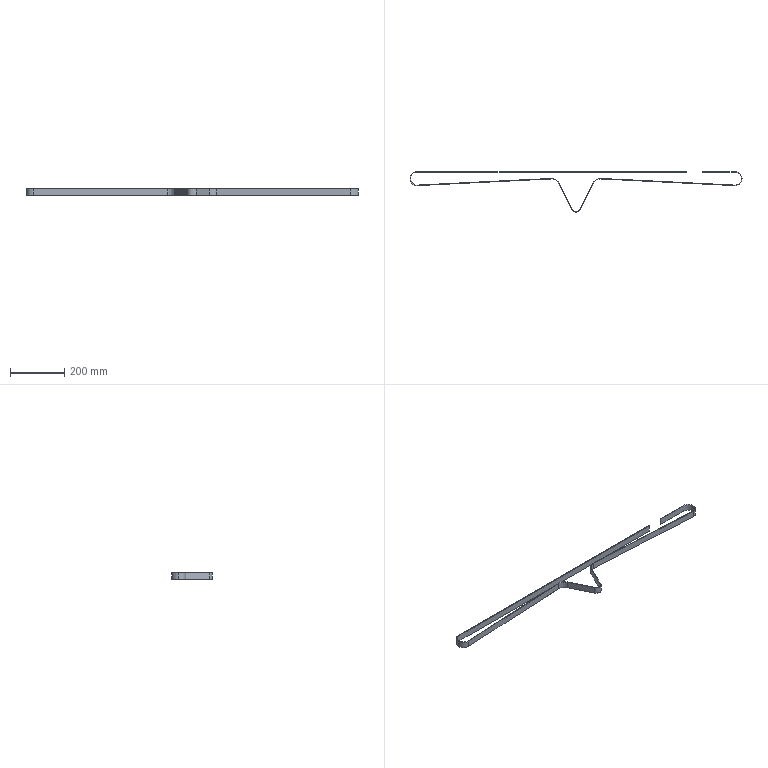Part | SolidWorks | features BaseBody 1 | 1 solid | 28 faces | box 1221 x 148.8 x 24 mm | volume 123601 mm3 | plane 16 | cylinder 12 | commonest cylinder face diameters 47 x3 51 x3 60 x2 64 x2 31 x1 35 x1
STEP:
#1=CARTESIAN_POINT('',(-1151.5,-71.7,12.));
#2=VERTEX_POINT('',#1);
#3=CARTESIAN_POINT('',(-1128.,-48.2,12.));
#4=VERTEX_POINT('',#3);
#5=CARTESIAN_POINT('',(-1128.,-71.7,12.));
#6=DIRECTION('',(0.,0.,-1.));
#7=DIRECTION('',(-1.,0.,0.));
#8=AXIS2_PLACEMENT_3D('',#5,#6,#7);
#9=CIRCLE('',#8,23.5);
#10=EDGE_CURVE('',#2,#4,#9,.T.);
#11=ORIENTED_EDGE('',*,*,#10,.F.);
#12=CARTESIAN_POINT('',(-1151.5,-71.7,-12.));
#13=VERTEX_POINT('',#12);
#14=CARTESIAN_POINT('',(-1151.5,-71.7,12.));
#15=DIRECTION('',(0.,0.,-1.));
#16=VECTOR('',#15,1000.);
#17=LINE('',#14,#16);
#18=EDGE_CURVE('',#2,#13,#17,.T.);
#19=ORIENTED_EDGE('',*,*,#18,.T.);
#20=CARTESIAN_POINT('',(-1128.,-48.2,-12.));
#21=VERTEX_POINT('',#20);
#22=CARTESIAN_POINT('',(-1128.,-71.7,-12.));
#23=DIRECTION('',(0.,0.,-1.));
#24=DIRECTION('',(-1.,0.,0.));
#25=AXIS2_PLACEMENT_3D('',#22,#23,#24);
#26=CIRCLE('',#25,23.5);
#27=EDGE_CURVE('',#13,#21,#26,.T.);
#28=ORIENTED_EDGE('',*,*,#27,.T.);
#29=CARTESIAN_POINT('',(-1128.,-48.2,12.));
#30=DIRECTION('',(0.,0.,-1.));
#31=VECTOR('',#30,1000.);
#32=LINE('',#29,#31);
#33=EDGE_CURVE('',#4,#21,#32,.T.);
#34=ORIENTED_EDGE('',*,*,#33,.F.);
#35=EDGE_LOOP('',(#11,#19,#28,#34));
#36=FACE_OUTER_BOUND('',#35,.T.);
#37=CARTESIAN_POINT('',(-1128.,-71.7,12.));
#38=DIRECTION('',(0.,0.,-1.));
#39=DIRECTION('',(-1.,0.,0.));
#40=AXIS2_PLACEMENT_3D('',#37,#38,#39);
#41=CYLINDRICAL_SURFACE('',#40,23.5);
#42=ADVANCED_FACE('',(#36),#41,.F.);
#43=CARTESIAN_POINT('',(-1153.5,-71.7,12.));
#44=VERTEX_POINT('',#43);
#45=CARTESIAN_POINT('',(-1126.726,-97.168,12.));
#46=VERTEX_POINT('',#45);
#47=CARTESIAN_POINT('',(-1128.,-71.7,12.));
#48=DIRECTION('',(0.,0.,1.));
#49=DIRECTION('',(1.,0.,0.));
#50=AXIS2_PLACEMENT_3D('',#47,#48,#49);
#51=CIRCLE('',#50,25.5);
#52=EDGE_CURVE('',#44,#46,#51,.T.);
#53=ORIENTED_EDGE('',*,*,#52,.F.);
#54=CARTESIAN_POINT('',(-1153.5,-71.7,-12.));
#55=VERTEX_POINT('',#54);
#56=CARTESIAN_POINT('',(-1153.5,-71.7,12.));
#57=DIRECTION('',(0.,0.,-1.));
#58=VECTOR('',#57,1000.);
#59=LINE('',#56,#58);
#60=EDGE_CURVE('',#44,#55,#59,.T.);
#61=ORIENTED_EDGE('',*,*,#60,.T.);
#62=CARTESIAN_POINT('',(-1126.726,-97.168,-12.));
#63=VERTEX_POINT('',#62);
#64=CARTESIAN_POINT('',(-1128.,-71.7,-12.));
#65=DIRECTION('',(0.,0.,1.));
#66=DIRECTION('',(1.,0.,0.));
#67=AXIS2_PLACEMENT_3D('',#64,#65,#66);
#68=CIRCLE('',#67,25.5);
#69=EDGE_CURVE('',#55,#63,#68,.T.);
#70=ORIENTED_EDGE('',*,*,#69,.T.);
#71=CARTESIAN_POINT('',(-1126.726,-97.168,12.));
#72=DIRECTION('',(0.,0.,-1.));
#73=VECTOR('',#72,1000.);
#74=LINE('',#71,#73);
#75=EDGE_CURVE('',#46,#63,#74,.T.);
#76=ORIENTED_EDGE('',*,*,#75,.F.);
#77=EDGE_LOOP('',(#53,#61,#70,#76));
#78=FACE_OUTER_BOUND('',#77,.T.);
#79=CARTESIAN_POINT('',(-1128.,-71.7,12.));
#80=DIRECTION('',(0.,0.,-1.));
#81=DIRECTION('',(-1.,0.,0.));
#82=AXIS2_PLACEMENT_3D('',#79,#80,#81);
#83=CYLINDRICAL_SURFACE('',#82,25.5);
#84=ADVANCED_FACE('',(#78),#83,.T.);
#85=CARTESIAN_POINT('',(-138.,-46.2,12.));
#86=VERTEX_POINT('',#85);
#87=CARTESIAN_POINT('',(-1128.,-46.2,12.));
#88=VERTEX_POINT('',#87);
#89=CARTESIAN_POINT('',(-1128.,-46.2,12.));
#90=DIRECTION('',(-1.,0.,0.));
#91=VECTOR('',#90,1000.);
#92=LINE('',#89,#91);
#93=EDGE_CURVE('',#86,#88,#92,.T.);
#94=ORIENTED_EDGE('',*,*,#93,.F.);
#95=CARTESIAN_POINT('',(-138.,-46.2,-12.));
#96=VERTEX_POINT('',#95);
#97=CARTESIAN_POINT('',(-138.,-46.2,12.));
#98=DIRECTION('',(0.,0.,1.));
#99=VECTOR('',#98,1000.);
#100=LINE('',#97,#99);
#101=EDGE_CURVE('',#96,#86,#100,.T.);
#102=ORIENTED_EDGE('',*,*,#101,.F.);
#103=CARTESIAN_POINT('',(-1128.,-46.2,-12.));
#104=VERTEX_POINT('',#103);
#105=CARTESIAN_POINT('',(-1128.,-46.2,-12.));
#106=DIRECTION('',(-1.,0.,0.));
#107=VECTOR('',#106,1000.);
#108=LINE('',#105,#107);
#109=EDGE_CURVE('',#96,#104,#108,.T.);
#110=ORIENTED_EDGE('',*,*,#109,.T.);
#111=CARTESIAN_POINT('',(-1128.,-46.2,12.));
#112=DIRECTION('',(0.,0.,-1.));
#113=VECTOR('',#112,1000.);
#114=LINE('',#111,#113);
#115=EDGE_CURVE('',#88,#104,#114,.T.);
#116=ORIENTED_EDGE('',*,*,#115,.F.);
#117=EDGE_LOOP('',(#94,#102,#110,#116));
#118=FACE_OUTER_BOUND('',#117,.T.);
#119=CARTESIAN_POINT('',(-1128.,-46.2,12.));
#120=DIRECTION('',(0.,-1.,0.));
#121=DIRECTION('',(0.,0.,-1.));
#122=AXIS2_PLACEMENT_3D('',#119,#120,#121);
#123=PLANE('',#122);
#124=ADVANCED_FACE('',(#118),#123,.F.);
#125=CARTESIAN_POINT('',(-138.,-48.2,12.));
#126=VERTEX_POINT('',#125);
#127=CARTESIAN_POINT('',(-138.,-48.2,-12.));
#128=VERTEX_POINT('',#127);
#129=CARTESIAN_POINT('',(-138.,-48.2,12.));
#130=DIRECTION('',(0.,0.,-1.));
#131=VECTOR('',#130,1000.);
#132=LINE('',#129,#131);
#133=EDGE_CURVE('',#126,#128,#132,.T.);
#134=ORIENTED_EDGE('',*,*,#133,.F.);
#135=CARTESIAN_POINT('',(-1128.,-48.2,12.));
#136=DIRECTION('',(1.,0.,0.));
#137=VECTOR('',#136,1000.);
#138=LINE('',#135,#137);
#139=EDGE_CURVE('',#4,#126,#138,.T.);
#140=ORIENTED_EDGE('',*,*,#139,.F.);
#141=ORIENTED_EDGE('',*,*,#33,.T.);
#142=CARTESIAN_POINT('',(-1128.,-48.2,-12.));
#143=DIRECTION('',(1.,0.,0.));
#144=VECTOR('',#143,1000.);
#145=LINE('',#142,#144);
#146=EDGE_CURVE('',#21,#128,#145,.T.);
#147=ORIENTED_EDGE('',*,*,#146,.T.);
#148=EDGE_LOOP('',(#134,#140,#141,#147));
#149=FACE_OUTER_BOUND('',#148,.T.);
#150=CARTESIAN_POINT('',(-1128.,-48.2,12.));
#151=DIRECTION('',(0.,-1.,0.));
#152=DIRECTION('',(0.,0.,-1.));
#153=AXIS2_PLACEMENT_3D('',#150,#151,#152);
#154=PLANE('',#153);
#155=ADVANCED_FACE('',(#149),#154,.T.);
#156=CARTESIAN_POINT('',(40.726,-97.168,-12.));
#157=VERTEX_POINT('',#156);
#158=CARTESIAN_POINT('',(42.,-46.2,-12.));
#159=VERTEX_POINT('',#158);
#160=CARTESIAN_POINT('',(42.,-71.7,-12.));
#161=DIRECTION('',(0.,0.,1.));
#162=DIRECTION('',(1.,0.,0.));
#163=AXIS2_PLACEMENT_3D('',#160,#161,#162);
#164=CIRCLE('',#163,25.5);
#165=EDGE_CURVE('',#157,#159,#164,.T.);
#166=ORIENTED_EDGE('',*,*,#165,.T.);
#167=CARTESIAN_POINT('',(42.,-46.2,12.));
#168=VERTEX_POINT('',#167);
#169=CARTESIAN_POINT('',(42.,-46.2,12.));
#170=DIRECTION('',(0.,0.,-1.));
#171=VECTOR('',#170,1000.);
#172=LINE('',#169,#171);
#173=EDGE_CURVE('',#168,#159,#172,.T.);
#174=ORIENTED_EDGE('',*,*,#173,.F.);
#175=CARTESIAN_POINT('',(40.726,-97.168,12.));
#176=VERTEX_POINT('',#175);
#177=CARTESIAN_POINT('',(42.,-71.7,12.));
#178=DIRECTION('',(0.,0.,1.));
#179=DIRECTION('',(1.,0.,0.));
#180=AXIS2_PLACEMENT_3D('',#177,#178,#179);
#181=CIRCLE('',#180,25.5);
#182=EDGE_CURVE('',#176,#168,#181,.T.);
#183=ORIENTED_EDGE('',*,*,#182,.F.);
#184=CARTESIAN_POINT('',(40.726,-97.168,12.));
#185=DIRECTION('',(0.,0.,-1.));
#186=VECTOR('',#185,1000.);
#187=LINE('',#184,#186);
#188=EDGE_CURVE('',#176,#157,#187,.T.);
#189=ORIENTED_EDGE('',*,*,#188,.T.);
#190=EDGE_LOOP('',(#166,#174,#183,#189));
#191=FACE_OUTER_BOUND('',#190,.T.);
#192=CARTESIAN_POINT('',(42.,-71.7,12.));
#193=DIRECTION('',(0.,0.,-1.));
#194=DIRECTION('',(-1.,0.,0.));
#195=AXIS2_PLACEMENT_3D('',#192,#193,#194);
#196=CYLINDRICAL_SURFACE('',#195,25.5);
#197=ADVANCED_FACE('',(#191),#196,.T.);
#198=CARTESIAN_POINT('',(-78.,-46.2,-12.));
#199=VERTEX_POINT('',#198);
#200=CARTESIAN_POINT('',(-1128.,-46.2,-12.));
#201=DIRECTION('',(-1.,0.,0.));
#202=VECTOR('',#201,1000.);
#203=LINE('',#200,#202);
#204=EDGE_CURVE('',#159,#199,#203,.T.);
#205=ORIENTED_EDGE('',*,*,#204,.T.);
#206=CARTESIAN_POINT('',(-78.,-46.2,12.));
#207=VERTEX_POINT('',#206);
#208=CARTESIAN_POINT('',(-78.,-46.2,12.));
#209=DIRECTION('',(0.,0.,-1.));
#210=VECTOR('',#209,1000.);
#211=LINE('',#208,#210);
#212=EDGE_CURVE('',#207,#199,#211,.T.);
#213=ORIENTED_EDGE('',*,*,#212,.F.);
#214=CARTESIAN_POINT('',(-1128.,-46.2,12.));
#215=DIRECTION('',(-1.,0.,0.));
#216=VECTOR('',#215,1000.);
#217=LINE('',#214,#216);
#218=EDGE_CURVE('',#168,#207,#217,.T.);
#219=ORIENTED_EDGE('',*,*,#218,.F.);
#220=ORIENTED_EDGE('',*,*,#173,.T.);
#221=EDGE_LOOP('',(#205,#213,#219,#220));
#222=FACE_OUTER_BOUND('',#221,.T.);
#223=CARTESIAN_POINT('',(-1128.,-46.2,12.));
#224=DIRECTION('',(0.,-1.,0.));
#225=DIRECTION('',(0.,0.,-1.));
#226=AXIS2_PLACEMENT_3D('',#223,#224,#225);
#227=PLANE('',#226);
#228=ADVANCED_FACE('',(#222),#227,.F.);
#229=ORIENTED_EDGE('',*,*,#60,.F.);
#230=CARTESIAN_POINT('',(-1128.,-71.7,12.));
#231=DIRECTION('',(0.,0.,1.));
#232=DIRECTION('',(1.,0.,0.));
#233=AXIS2_PLACEMENT_3D('',#230,#231,#232);
#234=CIRCLE('',#233,25.5);
#235=EDGE_CURVE('',#88,#44,#234,.T.);
#236=ORIENTED_EDGE('',*,*,#235,.F.);
#237=ORIENTED_EDGE('',*,*,#115,.T.);
#238=CARTESIAN_POINT('',(-1128.,-71.7,-12.));
#239=DIRECTION('',(0.,0.,1.));
#240=DIRECTION('',(1.,0.,0.));
#241=AXIS2_PLACEMENT_3D('',#238,#239,#240);
#242=CIRCLE('',#241,25.5);
#243=EDGE_CURVE('',#104,#55,#242,.T.);
#244=ORIENTED_EDGE('',*,*,#243,.T.);
#245=EDGE_LOOP('',(#229,#236,#237,#244));
#246=FACE_OUTER_BOUND('',#245,.T.);
#247=CARTESIAN_POINT('',(-1128.,-71.7,12.));
#248=DIRECTION('',(0.,0.,-1.));
#249=DIRECTION('',(-1.,0.,0.));
#250=AXIS2_PLACEMENT_3D('',#247,#248,#249);
#251=CYLINDRICAL_SURFACE('',#250,25.5);
#252=ADVANCED_FACE('',(#246),#251,.T.);
#253=CARTESIAN_POINT('',(-634.499,-72.537,-12.));
#254=VERTEX_POINT('',#253);
#255=CARTESIAN_POINT('',(-1126.726,-97.168,-12.));
#256=DIRECTION('',(0.9988,0.04998,0.));
#257=VECTOR('',#256,1000.);
#258=LINE('',#255,#257);
#259=EDGE_CURVE('',#63,#254,#258,.T.);
#260=ORIENTED_EDGE('',*,*,#259,.T.);
#261=CARTESIAN_POINT('',(-634.499,-72.537,12.));
#262=VERTEX_POINT('',#261);
#263=CARTESIAN_POINT('',(-634.499,-72.537,12.));
#264=DIRECTION('',(0.,0.,-1.));
#265=VECTOR('',#264,1000.);
#266=LINE('',#263,#265);
#267=EDGE_CURVE('',#262,#254,#266,.T.);
#268=ORIENTED_EDGE('',*,*,#267,.F.);
#269=CARTESIAN_POINT('',(-1126.726,-97.168,12.));
#270=DIRECTION('',(0.9988,0.04998,0.));
#271=VECTOR('',#270,1000.);
#272=LINE('',#269,#271);
#273=EDGE_CURVE('',#46,#262,#272,.T.);
#274=ORIENTED_EDGE('',*,*,#273,.F.);
#275=ORIENTED_EDGE('',*,*,#75,.T.);
#276=EDGE_LOOP('',(#260,#268,#274,#275));
#277=FACE_OUTER_BOUND('',#276,.T.);
#278=CARTESIAN_POINT('',(-1126.726,-97.168,12.));
#279=DIRECTION('',(-0.04998,0.9988,0.));
#280=DIRECTION('',(-0.9988,-0.04998,0.));
#281=AXIS2_PLACEMENT_3D('',#278,#279,#280);
#282=PLANE('',#281);
#283=ADVANCED_FACE('',(#277),#282,.F.);
#284=CARTESIAN_POINT('',(-606.1,-89.22,-12.));
#285=VERTEX_POINT('',#284);
#286=CARTESIAN_POINT('',(-633.,-102.5,-12.));
#287=DIRECTION('',(0.,0.,-1.));
#288=DIRECTION('',(1.,0.,0.));
#289=AXIS2_PLACEMENT_3D('',#286,#287,#288);
#290=CIRCLE('',#289,30.);
#291=EDGE_CURVE('',#254,#285,#290,.T.);
#292=ORIENTED_EDGE('',*,*,#291,.T.);
#293=CARTESIAN_POINT('',(-606.1,-89.22,12.));
#294=VERTEX_POINT('',#293);
#295=CARTESIAN_POINT('',(-606.1,-89.22,12.));
#296=DIRECTION('',(0.,0.,-1.));
#297=VECTOR('',#296,1000.);
#298=LINE('',#295,#297);
#299=EDGE_CURVE('',#294,#285,#298,.T.);
#300=ORIENTED_EDGE('',*,*,#299,.F.);
#301=CARTESIAN_POINT('',(-633.,-102.5,12.));
#302=DIRECTION('',(0.,0.,-1.));
#303=DIRECTION('',(1.,0.,0.));
#304=AXIS2_PLACEMENT_3D('',#301,#302,#303);
#305=CIRCLE('',#304,30.);
#306=EDGE_CURVE('',#262,#294,#305,.T.);
#307=ORIENTED_EDGE('',*,*,#306,.F.);
#308=ORIENTED_EDGE('',*,*,#267,.T.);
#309=EDGE_LOOP('',(#292,#300,#307,#308));
#310=FACE_OUTER_BOUND('',#309,.T.);
#311=CARTESIAN_POINT('',(-633.,-102.5,12.));
#312=DIRECTION('',(0.,0.,-1.));
#313=DIRECTION('',(-1.,0.,0.));
#314=AXIS2_PLACEMENT_3D('',#311,#312,#313);
#315=CYLINDRICAL_SURFACE('',#314,30.);
#316=ADVANCED_FACE('',(#310),#315,.F.);
#317=CARTESIAN_POINT('',(-558.692,-185.247,-12.));
#318=VERTEX_POINT('',#317);
#319=CARTESIAN_POINT('',(-606.1,-89.22,-12.));
#320=DIRECTION('',(0.4427,-0.8967,0.));
#321=VECTOR('',#320,1000.);
#322=LINE('',#319,#321);
#323=EDGE_CURVE('',#285,#318,#322,.T.);
#324=ORIENTED_EDGE('',*,*,#323,.T.);
#325=CARTESIAN_POINT('',(-558.692,-185.247,12.));
#326=VERTEX_POINT('',#325);
#327=CARTESIAN_POINT('',(-558.692,-185.247,12.));
#328=DIRECTION('',(0.,0.,-1.));
#329=VECTOR('',#328,1000.);
#330=LINE('',#327,#329);
#331=EDGE_CURVE('',#326,#318,#330,.T.);
#332=ORIENTED_EDGE('',*,*,#331,.F.);
#333=CARTESIAN_POINT('',(-606.1,-89.22,12.));
#334=DIRECTION('',(0.4427,-0.8967,0.));
#335=VECTOR('',#334,1000.);
#336=LINE('',#333,#335);
#337=EDGE_CURVE('',#294,#326,#336,.T.);
#338=ORIENTED_EDGE('',*,*,#337,.F.);
#339=ORIENTED_EDGE('',*,*,#299,.T.);
#340=EDGE_LOOP('',(#324,#332,#338,#339));
#341=FACE_OUTER_BOUND('',#340,.T.);
#342=CARTESIAN_POINT('',(-606.1,-89.22,12.));
#343=DIRECTION('',(0.8967,0.4427,0.));
#344=DIRECTION('',(-0.4427,0.8967,0.));
#345=AXIS2_PLACEMENT_3D('',#342,#343,#344);
#346=PLANE('',#345);
#347=ADVANCED_FACE('',(#341),#346,.F.);
#348=CARTESIAN_POINT('',(-527.308,-185.247,-12.));
#349=VERTEX_POINT('',#348);
#350=CARTESIAN_POINT('',(-543.,-177.5,-12.));
#351=DIRECTION('',(0.,0.,1.));
#352=DIRECTION('',(1.,0.,0.));
#353=AXIS2_PLACEMENT_3D('',#350,#351,#352);
#354=CIRCLE('',#353,17.5);
#355=EDGE_CURVE('',#318,#349,#354,.T.);
#356=ORIENTED_EDGE('',*,*,#355,.T.);
#357=CARTESIAN_POINT('',(-527.308,-185.247,12.));
#358=VERTEX_POINT('',#357);
#359=CARTESIAN_POINT('',(-527.308,-185.247,12.));
#360=DIRECTION('',(0.,0.,-1.));
#361=VECTOR('',#360,1000.);
#362=LINE('',#359,#361);
#363=EDGE_CURVE('',#358,#349,#362,.T.);
#364=ORIENTED_EDGE('',*,*,#363,.F.);
#365=CARTESIAN_POINT('',(-543.,-177.5,12.));
#366=DIRECTION('',(0.,0.,1.));
#367=DIRECTION('',(1.,0.,0.));
#368=AXIS2_PLACEMENT_3D('',#365,#366,#367);
#369=CIRCLE('',#368,17.5);
#370=EDGE_CURVE('',#326,#358,#369,.T.);
#371=ORIENTED_EDGE('',*,*,#370,.F.);
#372=ORIENTED_EDGE('',*,*,#331,.T.);
#373=EDGE_LOOP('',(#356,#364,#371,#372));
#374=FACE_OUTER_BOUND('',#373,.T.);
#375=CARTESIAN_POINT('',(-543.,-177.5,12.));
#376=DIRECTION('',(0.,0.,-1.));
#377=DIRECTION('',(-1.,0.,0.));
#378=AXIS2_PLACEMENT_3D('',#375,#376,#377);
#379=CYLINDRICAL_SURFACE('',#378,17.5);
#380=ADVANCED_FACE('',(#374),#379,.T.);
#381=CARTESIAN_POINT('',(-479.9,-89.22,-12.));
#382=VERTEX_POINT('',#381);
#383=CARTESIAN_POINT('',(-479.9,-89.22,-12.));
#384=DIRECTION('',(0.4427,0.8967,0.));
#385=VECTOR('',#384,1000.);
#386=LINE('',#383,#385);
#387=EDGE_CURVE('',#349,#382,#386,.T.);
#388=ORIENTED_EDGE('',*,*,#387,.T.);
#389=CARTESIAN_POINT('',(-479.9,-89.22,12.));
#390=VERTEX_POINT('',#389);
#391=CARTESIAN_POINT('',(-479.9,-89.22,12.));
#392=DIRECTION('',(0.,0.,-1.));
#393=VECTOR('',#392,1000.);
#394=LINE('',#391,#393);
#395=EDGE_CURVE('',#390,#382,#394,.T.);
#396=ORIENTED_EDGE('',*,*,#395,.F.);
#397=CARTESIAN_POINT('',(-479.9,-89.22,12.));
#398=DIRECTION('',(0.4427,0.8967,0.));
#399=VECTOR('',#398,1000.);
#400=LINE('',#397,#399);
#401=EDGE_CURVE('',#358,#390,#400,.T.);
#402=ORIENTED_EDGE('',*,*,#401,.F.);
#403=ORIENTED_EDGE('',*,*,#363,.T.);
#404=EDGE_LOOP('',(#388,#396,#402,#403));
#405=FACE_OUTER_BOUND('',#404,.T.);
#406=CARTESIAN_POINT('',(-479.9,-89.22,12.));
#407=DIRECTION('',(-0.8967,0.4427,0.));
#408=DIRECTION('',(-0.4427,-0.8967,0.));
#409=AXIS2_PLACEMENT_3D('',#406,#407,#408);
#410=PLANE('',#409);
#411=ADVANCED_FACE('',(#405),#410,.F.);
#412=CARTESIAN_POINT('',(-451.501,-72.537,-12.));
#413=VERTEX_POINT('',#412);
#414=CARTESIAN_POINT('',(-453.,-102.5,-12.));
#415=DIRECTION('',(0.,0.,-1.));
#416=DIRECTION('',(-1.,0.,0.));
#417=AXIS2_PLACEMENT_3D('',#414,#415,#416);
#418=CIRCLE('',#417,30.);
#419=EDGE_CURVE('',#382,#413,#418,.T.);
#420=ORIENTED_EDGE('',*,*,#419,.T.);
#421=CARTESIAN_POINT('',(-451.501,-72.537,12.));
#422=VERTEX_POINT('',#421);
#423=CARTESIAN_POINT('',(-451.501,-72.537,12.));
#424=DIRECTION('',(0.,0.,-1.));
#425=VECTOR('',#424,1000.);
#426=LINE('',#423,#425);
#427=EDGE_CURVE('',#422,#413,#426,.T.);
#428=ORIENTED_EDGE('',*,*,#427,.F.);
#429=CARTESIAN_POINT('',(-453.,-102.5,12.));
#430=DIRECTION('',(0.,0.,-1.));
#431=DIRECTION('',(-1.,0.,0.));
#432=AXIS2_PLACEMENT_3D('',#429,#430,#431);
#433=CIRCLE('',#432,30.);
#434=EDGE_CURVE('',#390,#422,#433,.T.);
#435=ORIENTED_EDGE('',*,*,#434,.F.);
#436=ORIENTED_EDGE('',*,*,#395,.T.);
#437=EDGE_LOOP('',(#420,#428,#435,#436));
#438=FACE_OUTER_BOUND('',#437,.T.);
#439=CARTESIAN_POINT('',(-453.,-102.5,12.));
#440=DIRECTION('',(0.,0.,-1.));
#441=DIRECTION('',(-1.,0.,0.));
#442=AXIS2_PLACEMENT_3D('',#439,#440,#441);
#443=CYLINDRICAL_SURFACE('',#442,30.);
#444=ADVANCED_FACE('',(#438),#443,.F.);
#445=CARTESIAN_POINT('',(40.726,-97.168,-12.));
#446=DIRECTION('',(0.9988,-0.04998,0.));
#447=VECTOR('',#446,1000.);
#448=LINE('',#445,#447);
#449=EDGE_CURVE('',#413,#157,#448,.T.);
#450=ORIENTED_EDGE('',*,*,#449,.T.);
#451=ORIENTED_EDGE('',*,*,#188,.F.);
#452=CARTESIAN_POINT('',(40.726,-97.168,12.));
#453=DIRECTION('',(0.9988,-0.04998,0.));
#454=VECTOR('',#453,1000.);
#455=LINE('',#452,#454);
#456=EDGE_CURVE('',#422,#176,#455,.T.);
#457=ORIENTED_EDGE('',*,*,#456,.F.);
#458=ORIENTED_EDGE('',*,*,#427,.T.);
#459=EDGE_LOOP('',(#450,#451,#457,#458));
#460=FACE_OUTER_BOUND('',#459,.T.);
#461=CARTESIAN_POINT('',(40.726,-97.168,12.));
#462=DIRECTION('',(0.04998,0.9988,0.));
#463=DIRECTION('',(-0.9988,0.04998,0.));
#464=AXIS2_PLACEMENT_3D('',#461,#462,#463);
#465=PLANE('',#464);
#466=ADVANCED_FACE('',(#460),#465,.F.);
#467=CARTESIAN_POINT('',(-138.,-56.2,12.));
#468=DIRECTION('',(0.,1.,0.));
#469=VECTOR('',#468,1000.);
#470=LINE('',#467,#469);
#471=EDGE_CURVE('',#126,#86,#470,.T.);
#472=ORIENTED_EDGE('',*,*,#471,.T.);
#473=ORIENTED_EDGE('',*,*,#93,.T.);
#474=ORIENTED_EDGE('',*,*,#235,.T.);
#475=ORIENTED_EDGE('',*,*,#52,.T.);
#476=ORIENTED_EDGE('',*,*,#273,.T.);
#477=ORIENTED_EDGE('',*,*,#306,.T.);
#478=ORIENTED_EDGE('',*,*,#337,.T.);
#479=ORIENTED_EDGE('',*,*,#370,.T.);
#480=ORIENTED_EDGE('',*,*,#401,.T.);
#481=ORIENTED_EDGE('',*,*,#434,.T.);
#482=ORIENTED_EDGE('',*,*,#456,.T.);
#483=ORIENTED_EDGE('',*,*,#182,.T.);
#484=ORIENTED_EDGE('',*,*,#218,.T.);
#485=CARTESIAN_POINT('',(-78.,-48.2,12.));
#486=VERTEX_POINT('',#485);
#487=CARTESIAN_POINT('',(-78.,-56.2,12.));
#488=DIRECTION('',(0.,1.,0.));
#489=VECTOR('',#488,1000.);
#490=LINE('',#487,#489);
#491=EDGE_CURVE('',#486,#207,#490,.T.);
#492=ORIENTED_EDGE('',*,*,#491,.F.);
#493=CARTESIAN_POINT('',(42.,-48.2,12.));
#494=VERTEX_POINT('',#493);
#495=CARTESIAN_POINT('',(-1128.,-48.2,12.));
#496=DIRECTION('',(1.,0.,0.));
#497=VECTOR('',#496,1000.);
#498=LINE('',#495,#497);
#499=EDGE_CURVE('',#486,#494,#498,.T.);
#500=ORIENTED_EDGE('',*,*,#499,.T.);
#501=CARTESIAN_POINT('',(40.826,-95.171,12.));
#502=VERTEX_POINT('',#501);
#503=CARTESIAN_POINT('',(42.,-71.7,12.));
#504=DIRECTION('',(0.,0.,-1.));
#505=DIRECTION('',(-1.,0.,0.));
#506=AXIS2_PLACEMENT_3D('',#503,#504,#505);
#507=CIRCLE('',#506,23.5);
#508=EDGE_CURVE('',#494,#502,#507,.T.);
#509=ORIENTED_EDGE('',*,*,#508,.T.);
#510=CARTESIAN_POINT('',(-451.401,-70.54,12.));
#511=VERTEX_POINT('',#510);
#512=CARTESIAN_POINT('',(40.826,-95.171,12.));
#513=DIRECTION('',(-0.9988,0.04998,0.));
#514=VECTOR('',#513,1000.);
#515=LINE('',#512,#514);
#516=EDGE_CURVE('',#502,#511,#515,.T.);
#517=ORIENTED_EDGE('',*,*,#516,.T.);
#518=CARTESIAN_POINT('',(-481.694,-88.334,12.));
#519=VERTEX_POINT('',#518);
#520=CARTESIAN_POINT('',(-453.,-102.5,12.));
#521=DIRECTION('',(0.,0.,1.));
#522=DIRECTION('',(-1.,0.,0.));
#523=AXIS2_PLACEMENT_3D('',#520,#521,#522);
#524=CIRCLE('',#523,32.);
#525=EDGE_CURVE('',#511,#519,#524,.T.);
#526=ORIENTED_EDGE('',*,*,#525,.T.);
#527=CARTESIAN_POINT('',(-529.101,-184.362,12.));
#528=VERTEX_POINT('',#527);
#529=CARTESIAN_POINT('',(-481.694,-88.334,12.));
#530=DIRECTION('',(-0.4427,-0.8967,0.));
#531=VECTOR('',#530,1000.);
#532=LINE('',#529,#531);
#533=EDGE_CURVE('',#519,#528,#532,.T.);
#534=ORIENTED_EDGE('',*,*,#533,.T.);
#535=CARTESIAN_POINT('',(-556.899,-184.362,12.));
#536=VERTEX_POINT('',#535);
#537=CARTESIAN_POINT('',(-543.,-177.5,12.));
#538=DIRECTION('',(0.,0.,-1.));
#539=DIRECTION('',(-1.,0.,0.));
#540=AXIS2_PLACEMENT_3D('',#537,#538,#539);
#541=CIRCLE('',#540,15.5);
#542=EDGE_CURVE('',#528,#536,#541,.T.);
#543=ORIENTED_EDGE('',*,*,#542,.T.);
#544=CARTESIAN_POINT('',(-604.306,-88.334,12.));
#545=VERTEX_POINT('',#544);
#546=CARTESIAN_POINT('',(-556.899,-184.362,12.));
#547=DIRECTION('',(-0.4427,0.8967,0.));
#548=VECTOR('',#547,1000.);
#549=LINE('',#546,#548);
#550=EDGE_CURVE('',#536,#545,#549,.T.);
#551=ORIENTED_EDGE('',*,*,#550,.T.);
#552=CARTESIAN_POINT('',(-634.599,-70.54,12.));
#553=VERTEX_POINT('',#552);
#554=CARTESIAN_POINT('',(-633.,-102.5,12.));
#555=DIRECTION('',(0.,0.,1.));
#556=DIRECTION('',(-1.,0.,0.));
#557=AXIS2_PLACEMENT_3D('',#554,#555,#556);
#558=CIRCLE('',#557,32.);
#559=EDGE_CURVE('',#545,#553,#558,.T.);
#560=ORIENTED_EDGE('',*,*,#559,.T.);
#561=CARTESIAN_POINT('',(-1126.826,-95.171,12.));
#562=VERTEX_POINT('',#561);
#563=CARTESIAN_POINT('',(-634.599,-70.54,12.));
#564=DIRECTION('',(-0.9988,-0.04998,0.));
#565=VECTOR('',#564,1000.);
#566=LINE('',#563,#565);
#567=EDGE_CURVE('',#553,#562,#566,.T.);
#568=ORIENTED_EDGE('',*,*,#567,.T.);
#569=CARTESIAN_POINT('',(-1128.,-71.7,12.));
#570=DIRECTION('',(0.,0.,-1.));
#571=DIRECTION('',(-1.,0.,0.));
#572=AXIS2_PLACEMENT_3D('',#569,#570,#571);
#573=CIRCLE('',#572,23.5);
#574=EDGE_CURVE('',#562,#2,#573,.T.);
#575=ORIENTED_EDGE('',*,*,#574,.T.);
#576=ORIENTED_EDGE('',*,*,#10,.T.);
#577=ORIENTED_EDGE('',*,*,#139,.T.);
#578=EDGE_LOOP('',(#472,#473,#474,#475,#476,#477,#478,#479,#480,#481,#482,#483,#484,#492,#500,#509,#517,#526,#534,#543,#551,#560,#568,#575,#576,#577));
#579=FACE_OUTER_BOUND('',#578,.T.);
#580=CARTESIAN_POINT('',(42.,-71.7,12.));
#581=DIRECTION('',(0.,0.,1.));
#582=DIRECTION('',(1.,0.,0.));
#583=AXIS2_PLACEMENT_3D('',#580,#581,#582);
#584=PLANE('',#583);
#585=ADVANCED_FACE('',(#579),#584,.T.);
#586=ORIENTED_EDGE('',*,*,#109,.F.);
#587=CARTESIAN_POINT('',(-138.,-56.2,-12.));
#588=DIRECTION('',(0.,1.,0.));
#589=VECTOR('',#588,1000.);
#590=LINE('',#587,#589);
#591=EDGE_CURVE('',#128,#96,#590,.T.);
#592=ORIENTED_EDGE('',*,*,#591,.F.);
#593=ORIENTED_EDGE('',*,*,#146,.F.);
#594=ORIENTED_EDGE('',*,*,#27,.F.);
#595=CARTESIAN_POINT('',(-1126.826,-95.171,-12.));
#596=VERTEX_POINT('',#595);
#597=CARTESIAN_POINT('',(-1128.,-71.7,-12.));
#598=DIRECTION('',(0.,0.,-1.));
#599=DIRECTION('',(-1.,0.,0.));
#600=AXIS2_PLACEMENT_3D('',#597,#598,#599);
#601=CIRCLE('',#600,23.5);
#602=EDGE_CURVE('',#596,#13,#601,.T.);
#603=ORIENTED_EDGE('',*,*,#602,.F.);
#604=CARTESIAN_POINT('',(-634.599,-70.54,-12.));
#605=VERTEX_POINT('',#604);
#606=CARTESIAN_POINT('',(-634.599,-70.54,-12.));
#607=DIRECTION('',(-0.9988,-0.04998,0.));
#608=VECTOR('',#607,1000.);
#609=LINE('',#606,#608);
#610=EDGE_CURVE('',#605,#596,#609,.T.);
#611=ORIENTED_EDGE('',*,*,#610,.F.);
#612=CARTESIAN_POINT('',(-604.306,-88.334,-12.));
#613=VERTEX_POINT('',#612);
#614=CARTESIAN_POINT('',(-633.,-102.5,-12.));
#615=DIRECTION('',(0.,0.,1.));
#616=DIRECTION('',(-1.,0.,0.));
#617=AXIS2_PLACEMENT_3D('',#614,#615,#616);
#618=CIRCLE('',#617,32.);
#619=EDGE_CURVE('',#613,#605,#618,.T.);
#620=ORIENTED_EDGE('',*,*,#619,.F.);
#621=CARTESIAN_POINT('',(-556.899,-184.362,-12.));
#622=VERTEX_POINT('',#621);
#623=CARTESIAN_POINT('',(-556.899,-184.362,-12.));
#624=DIRECTION('',(-0.4427,0.8967,0.));
#625=VECTOR('',#624,1000.);
#626=LINE('',#623,#625);
#627=EDGE_CURVE('',#622,#613,#626,.T.);
#628=ORIENTED_EDGE('',*,*,#627,.F.);
#629=CARTESIAN_POINT('',(-529.101,-184.362,-12.));
#630=VERTEX_POINT('',#629);
#631=CARTESIAN_POINT('',(-543.,-177.5,-12.));
#632=DIRECTION('',(0.,0.,-1.));
#633=DIRECTION('',(-1.,0.,0.));
#634=AXIS2_PLACEMENT_3D('',#631,#632,#633);
#635=CIRCLE('',#634,15.5);
#636=EDGE_CURVE('',#630,#622,#635,.T.);
#637=ORIENTED_EDGE('',*,*,#636,.F.);
#638=CARTESIAN_POINT('',(-481.694,-88.334,-12.));
#639=VERTEX_POINT('',#638);
#640=CARTESIAN_POINT('',(-481.694,-88.334,-12.));
#641=DIRECTION('',(-0.4427,-0.8967,0.));
#642=VECTOR('',#641,1000.);
#643=LINE('',#640,#642);
#644=EDGE_CURVE('',#639,#630,#643,.T.);
#645=ORIENTED_EDGE('',*,*,#644,.F.);
#646=CARTESIAN_POINT('',(-451.401,-70.54,-12.));
#647=VERTEX_POINT('',#646);
#648=CARTESIAN_POINT('',(-453.,-102.5,-12.));
#649=DIRECTION('',(0.,0.,1.));
#650=DIRECTION('',(-1.,0.,0.));
#651=AXIS2_PLACEMENT_3D('',#648,#649,#650);
#652=CIRCLE('',#651,32.);
#653=EDGE_CURVE('',#647,#639,#652,.T.);
#654=ORIENTED_EDGE('',*,*,#653,.F.);
#655=CARTESIAN_POINT('',(40.826,-95.171,-12.));
#656=VERTEX_POINT('',#655);
#657=CARTESIAN_POINT('',(40.826,-95.171,-12.));
#658=DIRECTION('',(-0.9988,0.04998,0.));
#659=VECTOR('',#658,1000.);
#660=LINE('',#657,#659);
#661=EDGE_CURVE('',#656,#647,#660,.T.);
#662=ORIENTED_EDGE('',*,*,#661,.F.);
#663=CARTESIAN_POINT('',(42.,-48.2,-12.));
#664=VERTEX_POINT('',#663);
#665=CARTESIAN_POINT('',(42.,-71.7,-12.));
#666=DIRECTION('',(0.,0.,-1.));
#667=DIRECTION('',(-1.,0.,0.));
#668=AXIS2_PLACEMENT_3D('',#665,#666,#667);
#669=CIRCLE('',#668,23.5);
#670=EDGE_CURVE('',#664,#656,#669,.T.);
#671=ORIENTED_EDGE('',*,*,#670,.F.);
#672=CARTESIAN_POINT('',(-78.,-48.2,-12.));
#673=VERTEX_POINT('',#672);
#674=CARTESIAN_POINT('',(-1128.,-48.2,-12.));
#675=DIRECTION('',(1.,0.,0.));
#676=VECTOR('',#675,1000.);
#677=LINE('',#674,#676);
#678=EDGE_CURVE('',#673,#664,#677,.T.);
#679=ORIENTED_EDGE('',*,*,#678,.F.);
#680=CARTESIAN_POINT('',(-78.,-56.2,-12.));
#681=DIRECTION('',(0.,1.,0.));
#682=VECTOR('',#681,1000.);
#683=LINE('',#680,#682);
#684=EDGE_CURVE('',#673,#199,#683,.T.);
#685=ORIENTED_EDGE('',*,*,#684,.T.);
#686=ORIENTED_EDGE('',*,*,#204,.F.);
#687=ORIENTED_EDGE('',*,*,#165,.F.);
#688=ORIENTED_EDGE('',*,*,#449,.F.);
#689=ORIENTED_EDGE('',*,*,#419,.F.);
#690=ORIENTED_EDGE('',*,*,#387,.F.);
#691=ORIENTED_EDGE('',*,*,#355,.F.);
#692=ORIENTED_EDGE('',*,*,#323,.F.);
#693=ORIENTED_EDGE('',*,*,#291,.F.);
#694=ORIENTED_EDGE('',*,*,#259,.F.);
#695=ORIENTED_EDGE('',*,*,#69,.F.);
#696=ORIENTED_EDGE('',*,*,#243,.F.);
#697=EDGE_LOOP('',(#586,#592,#593,#594,#603,#611,#620,#628,#637,#645,#654,#662,#671,#679,#685,#686,#687,#688,#689,#690,#691,#692,#693,#694,#695,#696));
#698=FACE_OUTER_BOUND('',#697,.T.);
#699=CARTESIAN_POINT('',(42.,-71.7,-12.));
#700=DIRECTION('',(0.,0.,1.));
#701=DIRECTION('',(1.,0.,0.));
#702=AXIS2_PLACEMENT_3D('',#699,#700,#701);
#703=PLANE('',#702);
#704=ADVANCED_FACE('',(#698),#703,.F.);
#705=CARTESIAN_POINT('',(42.,-48.2,12.));
#706=DIRECTION('',(0.,0.,-1.));
#707=VECTOR('',#706,1000.);
#708=LINE('',#705,#707);
#709=EDGE_CURVE('',#494,#664,#708,.T.);
#710=ORIENTED_EDGE('',*,*,#709,.T.);
#711=ORIENTED_EDGE('',*,*,#670,.T.);
#712=CARTESIAN_POINT('',(40.826,-95.171,12.));
#713=DIRECTION('',(0.,0.,-1.));
#714=VECTOR('',#713,1000.);
#715=LINE('',#712,#714);
#716=EDGE_CURVE('',#502,#656,#715,.T.);
#717=ORIENTED_EDGE('',*,*,#716,.F.);
#718=ORIENTED_EDGE('',*,*,#508,.F.);
#719=EDGE_LOOP('',(#710,#711,#717,#718));
#720=FACE_OUTER_BOUND('',#719,.T.);
#721=CARTESIAN_POINT('',(42.,-71.7,12.));
#722=DIRECTION('',(0.,0.,-1.));
#723=DIRECTION('',(-1.,0.,0.));
#724=AXIS2_PLACEMENT_3D('',#721,#722,#723);
#725=CYLINDRICAL_SURFACE('',#724,23.5);
#726=ADVANCED_FACE('',(#720),#725,.F.);
#727=CARTESIAN_POINT('',(-78.,-48.2,12.));
#728=DIRECTION('',(0.,0.,1.));
#729=VECTOR('',#728,1000.);
#730=LINE('',#727,#729);
#731=EDGE_CURVE('',#673,#486,#730,.T.);
#732=ORIENTED_EDGE('',*,*,#731,.F.);
#733=ORIENTED_EDGE('',*,*,#678,.T.);
#734=ORIENTED_EDGE('',*,*,#709,.F.);
#735=ORIENTED_EDGE('',*,*,#499,.F.);
#736=EDGE_LOOP('',(#732,#733,#734,#735));
#737=FACE_OUTER_BOUND('',#736,.T.);
#738=CARTESIAN_POINT('',(-1128.,-48.2,12.));
#739=DIRECTION('',(0.,-1.,0.));
#740=DIRECTION('',(0.,0.,-1.));
#741=AXIS2_PLACEMENT_3D('',#738,#739,#740);
#742=PLANE('',#741);
#743=ADVANCED_FACE('',(#737),#742,.T.);
#744=ORIENTED_EDGE('',*,*,#18,.F.);
#745=ORIENTED_EDGE('',*,*,#574,.F.);
#746=CARTESIAN_POINT('',(-1126.826,-95.171,12.));
#747=DIRECTION('',(0.,0.,-1.));
#748=VECTOR('',#747,1000.);
#749=LINE('',#746,#748);
#750=EDGE_CURVE('',#562,#596,#749,.T.);
#751=ORIENTED_EDGE('',*,*,#750,.T.);
#752=ORIENTED_EDGE('',*,*,#602,.T.);
#753=EDGE_LOOP('',(#744,#745,#751,#752));
#754=FACE_OUTER_BOUND('',#753,.T.);
#755=CARTESIAN_POINT('',(-1128.,-71.7,12.));
#756=DIRECTION('',(0.,0.,-1.));
#757=DIRECTION('',(-1.,0.,0.));
#758=AXIS2_PLACEMENT_3D('',#755,#756,#757);
#759=CYLINDRICAL_SURFACE('',#758,23.5);
#760=ADVANCED_FACE('',(#754),#759,.F.);
#761=CARTESIAN_POINT('',(-634.599,-70.54,12.));
#762=DIRECTION('',(0.,0.,-1.));
#763=VECTOR('',#762,1000.);
#764=LINE('',#761,#763);
#765=EDGE_CURVE('',#553,#605,#764,.T.);
#766=ORIENTED_EDGE('',*,*,#765,.T.);
#767=ORIENTED_EDGE('',*,*,#610,.T.);
#768=ORIENTED_EDGE('',*,*,#750,.F.);
#769=ORIENTED_EDGE('',*,*,#567,.F.);
#770=EDGE_LOOP('',(#766,#767,#768,#769));
#771=FACE_OUTER_BOUND('',#770,.T.);
#772=CARTESIAN_POINT('',(-1126.826,-95.171,12.));
#773=DIRECTION('',(-0.04998,0.9988,0.));
#774=DIRECTION('',(-0.9988,-0.04998,0.));
#775=AXIS2_PLACEMENT_3D('',#772,#773,#774);
#776=PLANE('',#775);
#777=ADVANCED_FACE('',(#771),#776,.T.);
#778=CARTESIAN_POINT('',(-604.306,-88.334,12.));
#779=DIRECTION('',(0.,0.,-1.));
#780=VECTOR('',#779,1000.);
#781=LINE('',#778,#780);
#782=EDGE_CURVE('',#545,#613,#781,.T.);
#783=ORIENTED_EDGE('',*,*,#782,.T.);
#784=ORIENTED_EDGE('',*,*,#619,.T.);
#785=ORIENTED_EDGE('',*,*,#765,.F.);
#786=ORIENTED_EDGE('',*,*,#559,.F.);
#787=EDGE_LOOP('',(#783,#784,#785,#786));
#788=FACE_OUTER_BOUND('',#787,.T.);
#789=CARTESIAN_POINT('',(-633.,-102.5,12.));
#790=DIRECTION('',(0.,0.,-1.));
#791=DIRECTION('',(-1.,0.,0.));
#792=AXIS2_PLACEMENT_3D('',#789,#790,#791);
#793=CYLINDRICAL_SURFACE('',#792,32.);
#794=ADVANCED_FACE('',(#788),#793,.T.);
#795=CARTESIAN_POINT('',(-556.899,-184.362,12.));
#796=DIRECTION('',(0.,0.,-1.));
#797=VECTOR('',#796,1000.);
#798=LINE('',#795,#797);
#799=EDGE_CURVE('',#536,#622,#798,.T.);
#800=ORIENTED_EDGE('',*,*,#799,.T.);
#801=ORIENTED_EDGE('',*,*,#627,.T.);
#802=ORIENTED_EDGE('',*,*,#782,.F.);
#803=ORIENTED_EDGE('',*,*,#550,.F.);
#804=EDGE_LOOP('',(#800,#801,#802,#803));
#805=FACE_OUTER_BOUND('',#804,.T.);
#806=CARTESIAN_POINT('',(-604.306,-88.334,12.));
#807=DIRECTION('',(0.8967,0.4427,0.));
#808=DIRECTION('',(-0.4427,0.8967,0.));
#809=AXIS2_PLACEMENT_3D('',#806,#807,#808);
#810=PLANE('',#809);
#811=ADVANCED_FACE('',(#805),#810,.T.);
#812=CARTESIAN_POINT('',(-529.101,-184.362,12.));
#813=DIRECTION('',(0.,0.,-1.));
#814=VECTOR('',#813,1000.);
#815=LINE('',#812,#814);
#816=EDGE_CURVE('',#528,#630,#815,.T.);
#817=ORIENTED_EDGE('',*,*,#816,.T.);
#818=ORIENTED_EDGE('',*,*,#636,.T.);
#819=ORIENTED_EDGE('',*,*,#799,.F.);
#820=ORIENTED_EDGE('',*,*,#542,.F.);
#821=EDGE_LOOP('',(#817,#818,#819,#820));
#822=FACE_OUTER_BOUND('',#821,.T.);
#823=CARTESIAN_POINT('',(-543.,-177.5,12.));
#824=DIRECTION('',(0.,0.,-1.));
#825=DIRECTION('',(-1.,0.,0.));
#826=AXIS2_PLACEMENT_3D('',#823,#824,#825);
#827=CYLINDRICAL_SURFACE('',#826,15.5);
#828=ADVANCED_FACE('',(#822),#827,.F.);
#829=CARTESIAN_POINT('',(-481.694,-88.334,12.));
#830=DIRECTION('',(0.,0.,-1.));
#831=VECTOR('',#830,1000.);
#832=LINE('',#829,#831);
#833=EDGE_CURVE('',#519,#639,#832,.T.);
#834=ORIENTED_EDGE('',*,*,#833,.T.);
#835=ORIENTED_EDGE('',*,*,#644,.T.);
#836=ORIENTED_EDGE('',*,*,#816,.F.);
#837=ORIENTED_EDGE('',*,*,#533,.F.);
#838=EDGE_LOOP('',(#834,#835,#836,#837));
#839=FACE_OUTER_BOUND('',#838,.T.);
#840=CARTESIAN_POINT('',(-481.694,-88.334,12.));
#841=DIRECTION('',(-0.8967,0.4427,0.));
#842=DIRECTION('',(-0.4427,-0.8967,0.));
#843=AXIS2_PLACEMENT_3D('',#840,#841,#842);
#844=PLANE('',#843);
#845=ADVANCED_FACE('',(#839),#844,.T.);
#846=CARTESIAN_POINT('',(-451.401,-70.54,12.));
#847=DIRECTION('',(0.,0.,-1.));
#848=VECTOR('',#847,1000.);
#849=LINE('',#846,#848);
#850=EDGE_CURVE('',#511,#647,#849,.T.);
#851=ORIENTED_EDGE('',*,*,#850,.T.);
#852=ORIENTED_EDGE('',*,*,#653,.T.);
#853=ORIENTED_EDGE('',*,*,#833,.F.);
#854=ORIENTED_EDGE('',*,*,#525,.F.);
#855=EDGE_LOOP('',(#851,#852,#853,#854));
#856=FACE_OUTER_BOUND('',#855,.T.);
#857=CARTESIAN_POINT('',(-453.,-102.5,12.));
#858=DIRECTION('',(0.,0.,-1.));
#859=DIRECTION('',(-1.,0.,0.));
#860=AXIS2_PLACEMENT_3D('',#857,#858,#859);
#861=CYLINDRICAL_SURFACE('',#860,32.);
#862=ADVANCED_FACE('',(#856),#861,.T.);
#863=ORIENTED_EDGE('',*,*,#716,.T.);
#864=ORIENTED_EDGE('',*,*,#661,.T.);
#865=ORIENTED_EDGE('',*,*,#850,.F.);
#866=ORIENTED_EDGE('',*,*,#516,.F.);
#867=EDGE_LOOP('',(#863,#864,#865,#866));
#868=FACE_OUTER_BOUND('',#867,.T.);
#869=CARTESIAN_POINT('',(40.826,-95.171,12.));
#870=DIRECTION('',(0.04998,0.9988,0.));
#871=DIRECTION('',(-0.9988,0.04998,0.));
#872=AXIS2_PLACEMENT_3D('',#869,#870,#871);
#873=PLANE('',#872);
#874=ADVANCED_FACE('',(#868),#873,.T.);
#875=ORIENTED_EDGE('',*,*,#731,.T.);
#876=ORIENTED_EDGE('',*,*,#491,.T.);
#877=ORIENTED_EDGE('',*,*,#212,.T.);
#878=ORIENTED_EDGE('',*,*,#684,.F.);
#879=EDGE_LOOP('',(#875,#876,#877,#878));
#880=FACE_OUTER_BOUND('',#879,.T.);
#881=CARTESIAN_POINT('',(-78.,-56.2,12.));
#882=DIRECTION('',(1.,0.,0.));
#883=DIRECTION('',(0.,0.,-1.));
#884=AXIS2_PLACEMENT_3D('',#881,#882,#883);
#885=PLANE('',#884);
#886=ADVANCED_FACE('',(#880),#885,.F.);
#887=ORIENTED_EDGE('',*,*,#133,.T.);
#888=ORIENTED_EDGE('',*,*,#591,.T.);
#889=ORIENTED_EDGE('',*,*,#101,.T.);
#890=ORIENTED_EDGE('',*,*,#471,.F.);
#891=EDGE_LOOP('',(#887,#888,#889,#890));
#892=FACE_OUTER_BOUND('',#891,.T.);
#893=CARTESIAN_POINT('',(-138.,-56.2,12.));
#894=DIRECTION('',(-1.,0.,0.));
#895=DIRECTION('',(0.,0.,1.));
#896=AXIS2_PLACEMENT_3D('',#893,#894,#895);
#897=PLANE('',#896);
#898=ADVANCED_FACE('',(#892),#897,.F.);
#899=CLOSED_SHELL('',(#42,#84,#124,#155,#197,#228,#252,#283,#316,#347,#380,#411,#444,#466,#585,#704,#726,#743,#760,#777,#794,#811,#828,#845,#862,#874,#886,#898));
#900=MANIFOLD_SOLID_BREP('',#899);
#901=CARTESIAN_POINT('',(0.,0.,0.));
#902=DIRECTION('',(0.,0.,1.));
#903=DIRECTION('',(1.,0.,0.));
#904=AXIS2_PLACEMENT_3D('',#901,#902,#903);
#905=(LENGTH_UNIT()NAMED_UNIT(*)SI_UNIT(.MILLI.,.METRE.));
#906=UNCERTAINTY_MEASURE_WITH_UNIT(LENGTH_MEASURE(0.00001),#905,'','');
#907=(NAMED_UNIT(*)PLANE_ANGLE_UNIT()SI_UNIT($,.RADIAN.));
#908=(NAMED_UNIT(*)SI_UNIT($,.STERADIAN.)SOLID_ANGLE_UNIT());
#909=(GEOMETRIC_REPRESENTATION_CONTEXT(3)GLOBAL_UNCERTAINTY_ASSIGNED_CONTEXT((#906))GLOBAL_UNIT_ASSIGNED_CONTEXT((#905,#907,#908))REPRESENTATION_CONTEXT('',''));
#910=ADVANCED_BREP_SHAPE_REPRESENTATION('',(#900,#904),#909);